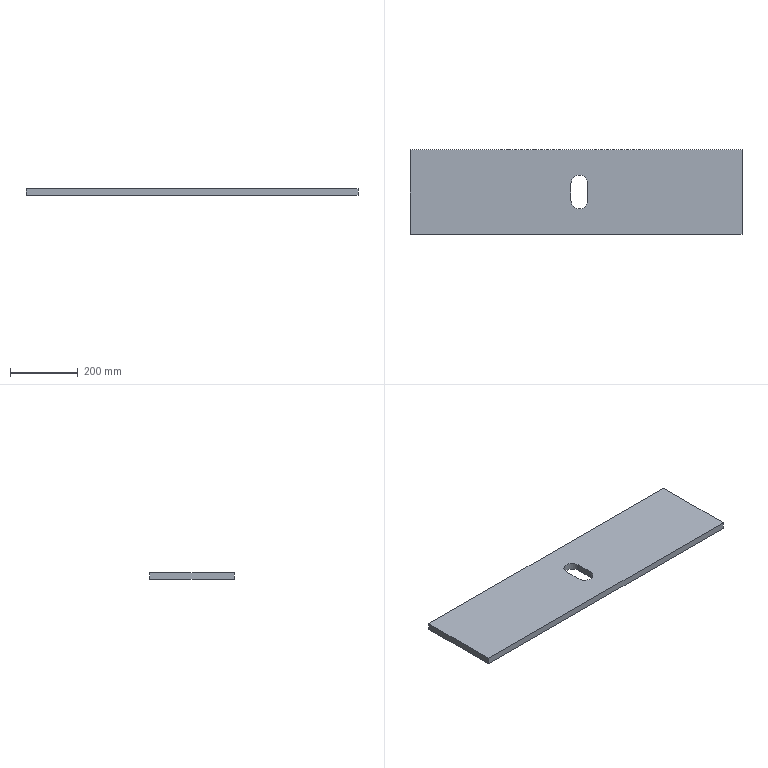Part | SolidWorks | features Extrusion 1 | 1 solid | 10 faces | box 980 x 250 x 20 mm | volume 4810730 mm3 | plane 8 | cylinder 2 | commonest cylinder face diameters 50 x2
STEP:
#1=CARTESIAN_POINT('',(12321.125,4637.824,20.));
#2=VERTEX_POINT('',#1);
#3=CARTESIAN_POINT('',(11341.125,4637.824,20.));
#4=VERTEX_POINT('',#3);
#5=CARTESIAN_POINT('',(11341.125,4637.824,20.));
#6=DIRECTION('',(-1.,0.,0.));
#7=VECTOR('',#6,1000.);
#8=LINE('',#5,#7);
#9=EDGE_CURVE('',#2,#4,#8,.T.);
#10=ORIENTED_EDGE('',*,*,#9,.T.);
#11=CARTESIAN_POINT('',(11341.125,4387.824,20.));
#12=VERTEX_POINT('',#11);
#13=CARTESIAN_POINT('',(11341.125,4637.824,20.));
#14=DIRECTION('',(0.,-1.,0.));
#15=VECTOR('',#14,1000.);
#16=LINE('',#13,#15);
#17=EDGE_CURVE('',#4,#12,#16,.T.);
#18=ORIENTED_EDGE('',*,*,#17,.T.);
#19=CARTESIAN_POINT('',(12321.125,4387.824,20.));
#20=VERTEX_POINT('',#19);
#21=CARTESIAN_POINT('',(11341.125,4387.824,20.));
#22=DIRECTION('',(1.,0.,0.));
#23=VECTOR('',#22,1000.);
#24=LINE('',#21,#23);
#25=EDGE_CURVE('',#12,#20,#24,.T.);
#26=ORIENTED_EDGE('',*,*,#25,.T.);
#27=CARTESIAN_POINT('',(12321.125,4637.824,20.));
#28=DIRECTION('',(0.,1.,0.));
#29=VECTOR('',#28,1000.);
#30=LINE('',#27,#29);
#31=EDGE_CURVE('',#20,#2,#30,.T.);
#32=ORIENTED_EDGE('',*,*,#31,.T.);
#33=EDGE_LOOP('',(#10,#18,#26,#32));
#34=FACE_OUTER_BOUND('',#33,.T.);
#35=CARTESIAN_POINT('',(11866.125,4537.824,20.));
#36=VERTEX_POINT('',#35);
#37=CARTESIAN_POINT('',(11816.125,4537.824,20.));
#38=VERTEX_POINT('',#37);
#39=CARTESIAN_POINT('',(11841.125,4537.824,20.));
#40=DIRECTION('',(0.,0.,1.));
#41=DIRECTION('',(1.,0.,0.));
#42=AXIS2_PLACEMENT_3D('',#39,#40,#41);
#43=CIRCLE('',#42,25.);
#44=EDGE_CURVE('',#36,#38,#43,.T.);
#45=ORIENTED_EDGE('',*,*,#44,.F.);
#46=CARTESIAN_POINT('',(11866.125,4487.824,20.));
#47=VERTEX_POINT('',#46);
#48=CARTESIAN_POINT('',(11866.125,4537.824,20.));
#49=DIRECTION('',(0.,1.,0.));
#50=VECTOR('',#49,1000.);
#51=LINE('',#48,#50);
#52=EDGE_CURVE('',#47,#36,#51,.T.);
#53=ORIENTED_EDGE('',*,*,#52,.F.);
#54=CARTESIAN_POINT('',(11816.125,4487.824,20.));
#55=VERTEX_POINT('',#54);
#56=CARTESIAN_POINT('',(11841.125,4487.824,20.));
#57=DIRECTION('',(0.,0.,1.));
#58=DIRECTION('',(1.,0.,0.));
#59=AXIS2_PLACEMENT_3D('',#56,#57,#58);
#60=CIRCLE('',#59,25.);
#61=EDGE_CURVE('',#55,#47,#60,.T.);
#62=ORIENTED_EDGE('',*,*,#61,.F.);
#63=CARTESIAN_POINT('',(11816.125,4537.824,20.));
#64=DIRECTION('',(0.,-1.,0.));
#65=VECTOR('',#64,1000.);
#66=LINE('',#63,#65);
#67=EDGE_CURVE('',#38,#55,#66,.T.);
#68=ORIENTED_EDGE('',*,*,#67,.F.);
#69=EDGE_LOOP('',(#45,#53,#62,#68));
#70=FACE_BOUND('',#69,.T.);
#71=CARTESIAN_POINT('',(0.,0.,20.));
#72=DIRECTION('',(0.,0.,-1.));
#73=DIRECTION('',(-1.,0.,0.));
#74=AXIS2_PLACEMENT_3D('',#71,#72,#73);
#75=PLANE('',#74);
#76=ADVANCED_FACE('',(#34,#70),#75,.F.);
#77=CARTESIAN_POINT('',(12321.125,4637.824,0.));
#78=VERTEX_POINT('',#77);
#79=CARTESIAN_POINT('',(11341.125,4637.824,0.));
#80=VERTEX_POINT('',#79);
#81=CARTESIAN_POINT('',(11341.125,4637.824,0.));
#82=DIRECTION('',(-1.,0.,0.));
#83=VECTOR('',#82,1000.);
#84=LINE('',#81,#83);
#85=EDGE_CURVE('',#78,#80,#84,.T.);
#86=ORIENTED_EDGE('',*,*,#85,.F.);
#87=CARTESIAN_POINT('',(12321.125,4387.824,0.));
#88=VERTEX_POINT('',#87);
#89=CARTESIAN_POINT('',(12321.125,4637.824,0.));
#90=DIRECTION('',(0.,1.,0.));
#91=VECTOR('',#90,1000.);
#92=LINE('',#89,#91);
#93=EDGE_CURVE('',#88,#78,#92,.T.);
#94=ORIENTED_EDGE('',*,*,#93,.F.);
#95=CARTESIAN_POINT('',(11341.125,4387.824,0.));
#96=VERTEX_POINT('',#95);
#97=CARTESIAN_POINT('',(11341.125,4387.824,0.));
#98=DIRECTION('',(1.,0.,0.));
#99=VECTOR('',#98,1000.);
#100=LINE('',#97,#99);
#101=EDGE_CURVE('',#96,#88,#100,.T.);
#102=ORIENTED_EDGE('',*,*,#101,.F.);
#103=CARTESIAN_POINT('',(11341.125,4637.824,0.));
#104=DIRECTION('',(0.,-1.,0.));
#105=VECTOR('',#104,1000.);
#106=LINE('',#103,#105);
#107=EDGE_CURVE('',#80,#96,#106,.T.);
#108=ORIENTED_EDGE('',*,*,#107,.F.);
#109=EDGE_LOOP('',(#86,#94,#102,#108));
#110=FACE_OUTER_BOUND('',#109,.T.);
#111=CARTESIAN_POINT('',(11866.125,4487.824,0.));
#112=VERTEX_POINT('',#111);
#113=CARTESIAN_POINT('',(11866.125,4537.824,0.));
#114=VERTEX_POINT('',#113);
#115=CARTESIAN_POINT('',(11866.125,4537.824,0.));
#116=DIRECTION('',(0.,1.,0.));
#117=VECTOR('',#116,1000.);
#118=LINE('',#115,#117);
#119=EDGE_CURVE('',#112,#114,#118,.T.);
#120=ORIENTED_EDGE('',*,*,#119,.T.);
#121=CARTESIAN_POINT('',(11816.125,4537.824,0.));
#122=VERTEX_POINT('',#121);
#123=CARTESIAN_POINT('',(11841.125,4537.824,0.));
#124=DIRECTION('',(0.,0.,1.));
#125=DIRECTION('',(1.,0.,0.));
#126=AXIS2_PLACEMENT_3D('',#123,#124,#125);
#127=CIRCLE('',#126,25.);
#128=EDGE_CURVE('',#114,#122,#127,.T.);
#129=ORIENTED_EDGE('',*,*,#128,.T.);
#130=CARTESIAN_POINT('',(11816.125,4487.824,0.));
#131=VERTEX_POINT('',#130);
#132=CARTESIAN_POINT('',(11816.125,4537.824,0.));
#133=DIRECTION('',(0.,-1.,0.));
#134=VECTOR('',#133,1000.);
#135=LINE('',#132,#134);
#136=EDGE_CURVE('',#122,#131,#135,.T.);
#137=ORIENTED_EDGE('',*,*,#136,.T.);
#138=CARTESIAN_POINT('',(11841.125,4487.824,0.));
#139=DIRECTION('',(0.,0.,1.));
#140=DIRECTION('',(1.,0.,0.));
#141=AXIS2_PLACEMENT_3D('',#138,#139,#140);
#142=CIRCLE('',#141,25.);
#143=EDGE_CURVE('',#131,#112,#142,.T.);
#144=ORIENTED_EDGE('',*,*,#143,.T.);
#145=EDGE_LOOP('',(#120,#129,#137,#144));
#146=FACE_BOUND('',#145,.T.);
#147=CARTESIAN_POINT('',(0.,0.,0.));
#148=DIRECTION('',(0.,0.,-1.));
#149=DIRECTION('',(-1.,0.,0.));
#150=AXIS2_PLACEMENT_3D('',#147,#148,#149);
#151=PLANE('',#150);
#152=ADVANCED_FACE('',(#110,#146),#151,.T.);
#153=ORIENTED_EDGE('',*,*,#85,.T.);
#154=CARTESIAN_POINT('',(11341.125,4637.824,20.));
#155=DIRECTION('',(0.,0.,-1.));
#156=VECTOR('',#155,1000.);
#157=LINE('',#154,#156);
#158=EDGE_CURVE('',#4,#80,#157,.T.);
#159=ORIENTED_EDGE('',*,*,#158,.F.);
#160=ORIENTED_EDGE('',*,*,#9,.F.);
#161=CARTESIAN_POINT('',(12321.125,4637.824,20.));
#162=DIRECTION('',(0.,0.,-1.));
#163=VECTOR('',#162,1000.);
#164=LINE('',#161,#163);
#165=EDGE_CURVE('',#2,#78,#164,.T.);
#166=ORIENTED_EDGE('',*,*,#165,.T.);
#167=EDGE_LOOP('',(#153,#159,#160,#166));
#168=FACE_OUTER_BOUND('',#167,.T.);
#169=CARTESIAN_POINT('',(11341.125,4637.824,20.));
#170=DIRECTION('',(0.,-1.,0.));
#171=DIRECTION('',(0.,0.,-1.));
#172=AXIS2_PLACEMENT_3D('',#169,#170,#171);
#173=PLANE('',#172);
#174=ADVANCED_FACE('',(#168),#173,.F.);
#175=ORIENTED_EDGE('',*,*,#107,.T.);
#176=CARTESIAN_POINT('',(11341.125,4387.824,20.));
#177=DIRECTION('',(0.,0.,-1.));
#178=VECTOR('',#177,1000.);
#179=LINE('',#176,#178);
#180=EDGE_CURVE('',#12,#96,#179,.T.);
#181=ORIENTED_EDGE('',*,*,#180,.F.);
#182=ORIENTED_EDGE('',*,*,#17,.F.);
#183=ORIENTED_EDGE('',*,*,#158,.T.);
#184=EDGE_LOOP('',(#175,#181,#182,#183));
#185=FACE_OUTER_BOUND('',#184,.T.);
#186=CARTESIAN_POINT('',(11341.125,4637.824,20.));
#187=DIRECTION('',(1.,0.,0.));
#188=DIRECTION('',(0.,1.,0.));
#189=AXIS2_PLACEMENT_3D('',#186,#187,#188);
#190=PLANE('',#189);
#191=ADVANCED_FACE('',(#185),#190,.F.);
#192=ORIENTED_EDGE('',*,*,#101,.T.);
#193=CARTESIAN_POINT('',(12321.125,4387.824,20.));
#194=DIRECTION('',(0.,0.,-1.));
#195=VECTOR('',#194,1000.);
#196=LINE('',#193,#195);
#197=EDGE_CURVE('',#20,#88,#196,.T.);
#198=ORIENTED_EDGE('',*,*,#197,.F.);
#199=ORIENTED_EDGE('',*,*,#25,.F.);
#200=ORIENTED_EDGE('',*,*,#180,.T.);
#201=EDGE_LOOP('',(#192,#198,#199,#200));
#202=FACE_OUTER_BOUND('',#201,.T.);
#203=CARTESIAN_POINT('',(11341.125,4387.824,20.));
#204=DIRECTION('',(0.,1.,0.));
#205=DIRECTION('',(0.,0.,1.));
#206=AXIS2_PLACEMENT_3D('',#203,#204,#205);
#207=PLANE('',#206);
#208=ADVANCED_FACE('',(#202),#207,.F.);
#209=ORIENTED_EDGE('',*,*,#93,.T.);
#210=ORIENTED_EDGE('',*,*,#165,.F.);
#211=ORIENTED_EDGE('',*,*,#31,.F.);
#212=ORIENTED_EDGE('',*,*,#197,.T.);
#213=EDGE_LOOP('',(#209,#210,#211,#212));
#214=FACE_OUTER_BOUND('',#213,.T.);
#215=CARTESIAN_POINT('',(12321.125,4637.824,20.));
#216=DIRECTION('',(-1.,0.,0.));
#217=DIRECTION('',(0.,0.,1.));
#218=AXIS2_PLACEMENT_3D('',#215,#216,#217);
#219=PLANE('',#218);
#220=ADVANCED_FACE('',(#214),#219,.F.);
#221=ORIENTED_EDGE('',*,*,#128,.F.);
#222=CARTESIAN_POINT('',(11866.125,4537.824,20.));
#223=DIRECTION('',(0.,0.,-1.));
#224=VECTOR('',#223,1000.);
#225=LINE('',#222,#224);
#226=EDGE_CURVE('',#36,#114,#225,.T.);
#227=ORIENTED_EDGE('',*,*,#226,.F.);
#228=ORIENTED_EDGE('',*,*,#44,.T.);
#229=CARTESIAN_POINT('',(11816.125,4537.824,20.));
#230=DIRECTION('',(0.,0.,-1.));
#231=VECTOR('',#230,1000.);
#232=LINE('',#229,#231);
#233=EDGE_CURVE('',#38,#122,#232,.T.);
#234=ORIENTED_EDGE('',*,*,#233,.T.);
#235=EDGE_LOOP('',(#221,#227,#228,#234));
#236=FACE_OUTER_BOUND('',#235,.T.);
#237=CARTESIAN_POINT('',(11841.125,4537.824,20.));
#238=DIRECTION('',(0.,0.,-1.));
#239=DIRECTION('',(-1.,0.,0.));
#240=AXIS2_PLACEMENT_3D('',#237,#238,#239);
#241=CYLINDRICAL_SURFACE('',#240,25.);
#242=ADVANCED_FACE('',(#236),#241,.F.);
#243=ORIENTED_EDGE('',*,*,#136,.F.);
#244=ORIENTED_EDGE('',*,*,#233,.F.);
#245=ORIENTED_EDGE('',*,*,#67,.T.);
#246=CARTESIAN_POINT('',(11816.125,4487.824,20.));
#247=DIRECTION('',(0.,0.,-1.));
#248=VECTOR('',#247,1000.);
#249=LINE('',#246,#248);
#250=EDGE_CURVE('',#55,#131,#249,.T.);
#251=ORIENTED_EDGE('',*,*,#250,.T.);
#252=EDGE_LOOP('',(#243,#244,#245,#251));
#253=FACE_OUTER_BOUND('',#252,.T.);
#254=CARTESIAN_POINT('',(11816.125,4537.824,20.));
#255=DIRECTION('',(1.,0.,0.));
#256=DIRECTION('',(0.,0.,-1.));
#257=AXIS2_PLACEMENT_3D('',#254,#255,#256);
#258=PLANE('',#257);
#259=ADVANCED_FACE('',(#253),#258,.T.);
#260=ORIENTED_EDGE('',*,*,#143,.F.);
#261=ORIENTED_EDGE('',*,*,#250,.F.);
#262=ORIENTED_EDGE('',*,*,#61,.T.);
#263=CARTESIAN_POINT('',(11866.125,4487.824,20.));
#264=DIRECTION('',(0.,0.,-1.));
#265=VECTOR('',#264,1000.);
#266=LINE('',#263,#265);
#267=EDGE_CURVE('',#47,#112,#266,.T.);
#268=ORIENTED_EDGE('',*,*,#267,.T.);
#269=EDGE_LOOP('',(#260,#261,#262,#268));
#270=FACE_OUTER_BOUND('',#269,.T.);
#271=CARTESIAN_POINT('',(11841.125,4487.824,20.));
#272=DIRECTION('',(0.,0.,-1.));
#273=DIRECTION('',(-1.,0.,0.));
#274=AXIS2_PLACEMENT_3D('',#271,#272,#273);
#275=CYLINDRICAL_SURFACE('',#274,25.);
#276=ADVANCED_FACE('',(#270),#275,.F.);
#277=ORIENTED_EDGE('',*,*,#119,.F.);
#278=ORIENTED_EDGE('',*,*,#267,.F.);
#279=ORIENTED_EDGE('',*,*,#52,.T.);
#280=ORIENTED_EDGE('',*,*,#226,.T.);
#281=EDGE_LOOP('',(#277,#278,#279,#280));
#282=FACE_OUTER_BOUND('',#281,.T.);
#283=CARTESIAN_POINT('',(11866.125,4537.824,20.));
#284=DIRECTION('',(-1.,0.,0.));
#285=DIRECTION('',(0.,0.,1.));
#286=AXIS2_PLACEMENT_3D('',#283,#284,#285);
#287=PLANE('',#286);
#288=ADVANCED_FACE('',(#282),#287,.T.);
#289=CLOSED_SHELL('',(#76,#152,#174,#191,#208,#220,#242,#259,#276,#288));
#290=MANIFOLD_SOLID_BREP('',#289);
#291=CARTESIAN_POINT('',(0.,0.,0.));
#292=DIRECTION('',(0.,0.,1.));
#293=DIRECTION('',(1.,0.,0.));
#294=AXIS2_PLACEMENT_3D('',#291,#292,#293);
#295=(LENGTH_UNIT()NAMED_UNIT(*)SI_UNIT(.MILLI.,.METRE.));
#296=UNCERTAINTY_MEASURE_WITH_UNIT(LENGTH_MEASURE(0.00001),#295,'','');
#297=(NAMED_UNIT(*)PLANE_ANGLE_UNIT()SI_UNIT($,.RADIAN.));
#298=(NAMED_UNIT(*)SI_UNIT($,.STERADIAN.)SOLID_ANGLE_UNIT());
#299=(GEOMETRIC_REPRESENTATION_CONTEXT(3)GLOBAL_UNCERTAINTY_ASSIGNED_CONTEXT((#296))GLOBAL_UNIT_ASSIGNED_CONTEXT((#295,#297,#298))REPRESENTATION_CONTEXT('',''));
#300=ADVANCED_BREP_SHAPE_REPRESENTATION('',(#290,#294),#299);